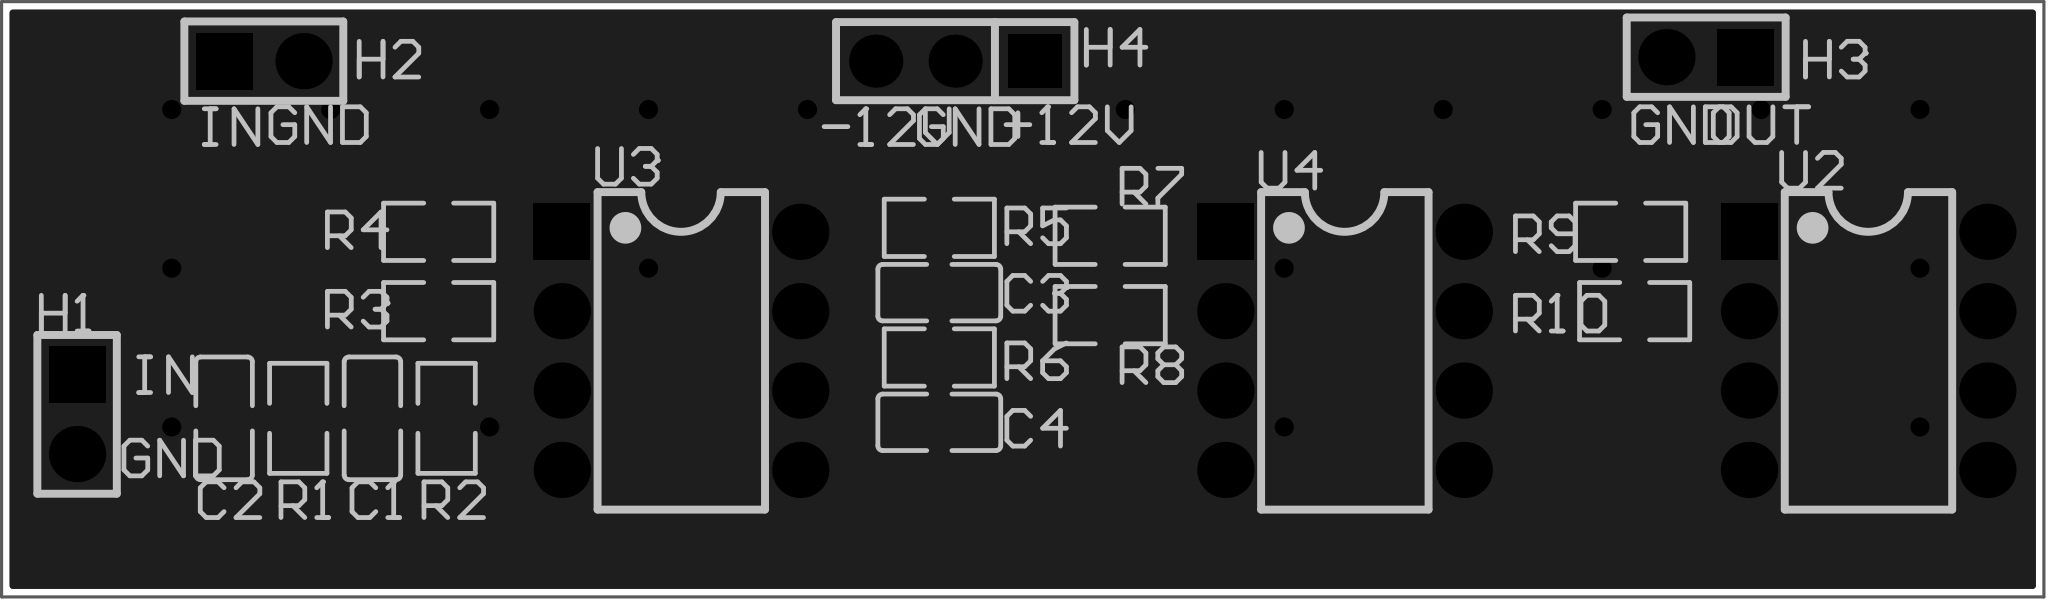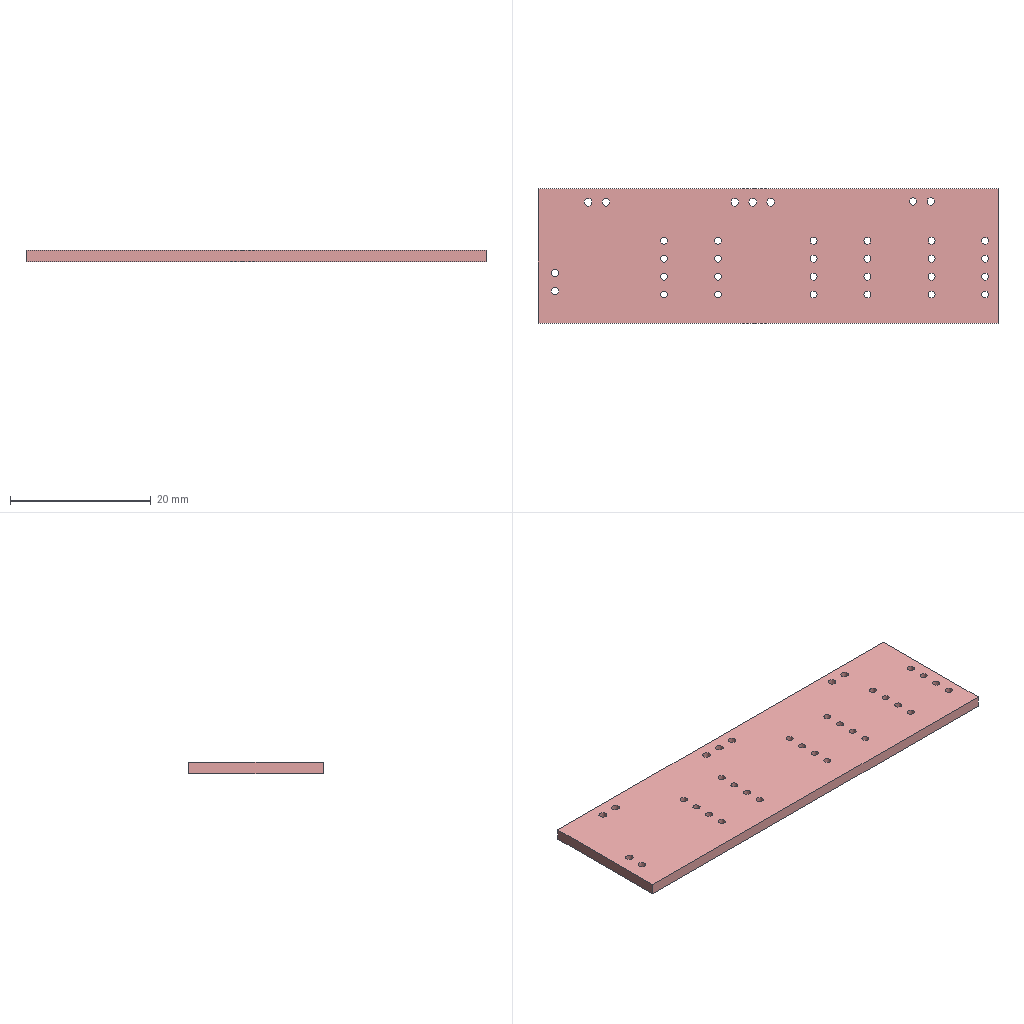Circuit board layout | Altium Designer | box 65.3 x 19 x 1.6 mm
Layer stack:
# Altium Designer layer stack of  (unit mm; dielectric type: 0 none, 1 core, 2 prepreg, 3 surface material)
index,name,kind,layer,copper_thickness_mm,dielectric_type,dielectric_thickness_mm,dielectric_material,dielectric_constant
0,Top Paste Mask Layer,other,,,,,,
1,Top Silkscreen Layer,other,,,,,,
2,Top Solder Mask Layer,dielectric,,,3,0.01,,3.3
3,Top Layer,copper,Top Layer,0.035,,,,
4,Dielectric1,dielectric,,,3,1.51,FR4,4.5
5,Bottom Layer,copper,Bottom Layer,0.035,,,,
6,Bottom Solder Mask Layer,dielectric,,,3,0.01,,3.3
7,Bottom Silkscreen Layer,other,,,,,,
8,Bottom Paste Mask Layer,other,,,,,,
# drill layer pairs: low layer,high layer
drill_pair,Top Layer,Bottom Layer
Part placement:
Designator,Comment,Layer,Footprint,Center-X(mm),Center-Y(mm),Rotation
C1,10uF,TopLayer,C0805,90.72,87.376,90
C2,10uF,TopLayer,C0805,85.979,87.376,270
C3,1nF,TopLayer,C0805,108.839,91.398,0
C4,1nF,TopLayer,C0805,108.839,87.249,180
H1,,TopLayer,HDR-TH_2P-P2.54-V-M-1,81.28,87.503,270
H2,,TopLayer,HDR-TH_2P-P2.54-V-M-1,87.249,98.806,0
H3,,TopLayer,HDR-TH_2P-P2.54-V-M-1,133.35,98.933,180
H4,,TopLayer,HDR-TH_3P-P2.54-V-M,109.347,98.806,180
R1,2.6K,TopLayer,R0805,88.35,87.376,270
R2,2.6K,TopLayer,R0805,93.091,87.376,90
R3,10K,TopLayer,R0805,92.837,90.805,0
R4,10K,TopLayer,R0805,92.837,93.345,180
R5,5.1K,TopLayer,R0805,108.839,93.472,0
R6,5.1K,TopLayer,R0805,108.839,89.323,180
R7,10K,TopLayer,R0805,114.3,93.218,180
R8,10K,TopLayer,R0805,114.3,90.678,0
R9,24K,TopLayer,R0805,130.937,93.345,180
R10,1K,TopLayer,R0805,131.064,90.805,0
U3,LM358AD,TopLayer,PDIP-8_L9.5-W6.4-P2.54-LS7.6-BL,100.584,89.535,270
U2,LM358AD,TopLayer,PDIP-8_L9.5-W6.4-P2.54-LS7.6-BL,138.53,89.535,270
U4,LM358AD,TopLayer,PDIP-8_L9.5-W6.4-P2.54-LS7.6-BL,121.793,89.535,270
Pad and via stacks:
# Altium Designer via and pad stacks of  (unit mm). Each distinct definition once, with the count of objects using it.
# via: kind,start_layer,end_layer,hole_mm,diameter_mm,mode(0 simple;1 top-mid-bottom;2 full stack),diameter_per_layer,count,example_net
# pad: kind,layer,hole_mm,hole_type(0 round;1 square;2 slot),plating,top_size,top_shape(1 round;2 rect;3 octagon;9 rounded rect),mid_size,bottom_size,mode,footprint,size_per_layer,count,example
pad,Top Layer,0,0,plated,1.41x1.35,2,1.41x1.35,1.41x1.35,0,C0805,,8,C1.2
pad,Top Layer,0,0,plated,1.133x1.377,2,1.133x1.377,1.133x1.377,0,R0805,,20,R1.2
pad,Multi-Layer,1.1,0,plated,1.8x1.8,1,1.8x1.8,1.8x1.8,0,HDR-TH_2P-P2.54-V-M-1,,3,H1.2
pad,Multi-Layer,1.1,0,plated,1.8x1.8,2,1.8x1.8,1.8x1.8,0,HDR-TH_2P-P2.54-V-M-1,,3,H1.1
pad,Multi-Layer,1.1,0,plated,1.7x1.7,2,1.7x1.7,1.7x1.7,0,HDR-TH_3P-P2.54-V-M,,1,H4.1
pad,Multi-Layer,1.1,0,plated,1.7x1.7,1,1.7x1.7,1.7x1.7,0,HDR-TH_3P-P2.54-V-M,,2,H4.2
pad,Multi-Layer,1,0,plated,1.8x1.8,1,1.8x1.8,1.8x1.8,0,PDIP-8_L9.5-W6.4-P2.54-LS7.6-BL,,21,U3.8
pad,Multi-Layer,1,0,plated,1.8x1.8,2,1.8x1.8,1.8x1.8,0,PDIP-8_L9.5-W6.4-P2.54-LS7.6-BL,,3,U3.1
via,Top Layer,Bottom Layer,0.3048,0.61,0,,20,GND
Copper pours:
name,layer,net,type(0 solid;1 hatched;2 none)
Top Layer-GND,Top Layer,GND,0
Bottom Layer-GND,Bottom Layer,GND,0